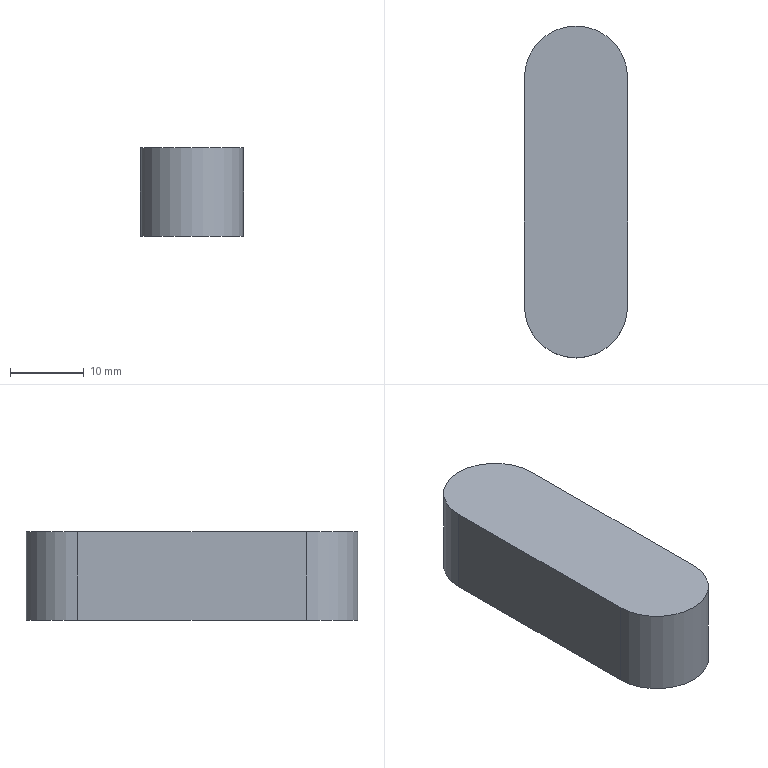Part | NX | features DATUM_CSYS 2, EXTRUDE 1, LINKED_FACE 1, SKETCH 1 | 1 solid | 6 faces | box 14 x 45 x 12 mm | volume 7055 mm3 | plane 4 | cylinder 2 | commonest cylinder face diameters 14 x2
STEP:
#1=CARTESIAN_POINT('',(35.,10.5,34.));
#2=VERTEX_POINT('',#1);
#3=CARTESIAN_POINT('',(35.,-20.5,34.));
#4=VERTEX_POINT('',#3);
#5=CARTESIAN_POINT('',(35.,10.5,34.));
#6=DIRECTION('',(0.,-1.,0.));
#7=VECTOR('',#6,1000.);
#8=LINE('',#5,#7);
#9=EDGE_CURVE('',#2,#4,#8,.T.);
#10=ORIENTED_EDGE('',*,*,#9,.T.);
#11=CARTESIAN_POINT('',(35.,-20.5,46.));
#12=VERTEX_POINT('',#11);
#13=CARTESIAN_POINT('',(35.,-20.5,46.));
#14=DIRECTION('',(0.,0.,-1.));
#15=VECTOR('',#14,1000.);
#16=LINE('',#13,#15);
#17=EDGE_CURVE('',#12,#4,#16,.T.);
#18=ORIENTED_EDGE('',*,*,#17,.F.);
#19=CARTESIAN_POINT('',(35.,10.5,46.));
#20=VERTEX_POINT('',#19);
#21=CARTESIAN_POINT('',(35.,10.5,46.));
#22=DIRECTION('',(0.,-1.,0.));
#23=VECTOR('',#22,1000.);
#24=LINE('',#21,#23);
#25=EDGE_CURVE('',#20,#12,#24,.T.);
#26=ORIENTED_EDGE('',*,*,#25,.F.);
#27=CARTESIAN_POINT('',(35.,10.5,46.));
#28=DIRECTION('',(0.,0.,-1.));
#29=VECTOR('',#28,1000.);
#30=LINE('',#27,#29);
#31=EDGE_CURVE('',#20,#2,#30,.T.);
#32=ORIENTED_EDGE('',*,*,#31,.T.);
#33=EDGE_LOOP('',(#10,#18,#26,#32));
#34=FACE_BOUND('',#33,.T.);
#35=CARTESIAN_POINT('',(35.,10.5,46.));
#36=DIRECTION('',(1.,0.,0.));
#37=DIRECTION('',(0.,1.,0.));
#38=AXIS2_PLACEMENT_3D('',#35,#36,#37);
#39=PLANE('',#38);
#40=ADVANCED_FACE('',(#34),#39,.F.);
#41=CARTESIAN_POINT('',(49.,-20.5,34.));
#42=VERTEX_POINT('',#41);
#43=CARTESIAN_POINT('',(42.,-20.5,34.));
#44=DIRECTION('',(0.,0.,1.));
#45=DIRECTION('',(-1.,0.,0.));
#46=AXIS2_PLACEMENT_3D('',#43,#44,#45);
#47=CIRCLE('',#46,7.);
#48=EDGE_CURVE('',#4,#42,#47,.T.);
#49=ORIENTED_EDGE('',*,*,#48,.T.);
#50=CARTESIAN_POINT('',(49.,-20.5,46.));
#51=VERTEX_POINT('',#50);
#52=CARTESIAN_POINT('',(49.,-20.5,46.));
#53=DIRECTION('',(0.,0.,-1.));
#54=VECTOR('',#53,1000.);
#55=LINE('',#52,#54);
#56=EDGE_CURVE('',#51,#42,#55,.T.);
#57=ORIENTED_EDGE('',*,*,#56,.F.);
#58=CARTESIAN_POINT('',(42.,-20.5,46.));
#59=DIRECTION('',(0.,0.,1.));
#60=DIRECTION('',(-1.,0.,0.));
#61=AXIS2_PLACEMENT_3D('',#58,#59,#60);
#62=CIRCLE('',#61,7.);
#63=EDGE_CURVE('',#12,#51,#62,.T.);
#64=ORIENTED_EDGE('',*,*,#63,.F.);
#65=ORIENTED_EDGE('',*,*,#17,.T.);
#66=EDGE_LOOP('',(#49,#57,#64,#65));
#67=FACE_BOUND('',#66,.T.);
#68=CARTESIAN_POINT('',(42.,-20.5,46.));
#69=DIRECTION('',(0.,0.,-1.));
#70=DIRECTION('',(-1.,0.,0.));
#71=AXIS2_PLACEMENT_3D('',#68,#69,#70);
#72=CYLINDRICAL_SURFACE('',#71,7.);
#73=ADVANCED_FACE('',(#67),#72,.T.);
#74=CARTESIAN_POINT('',(49.,10.5,34.));
#75=VERTEX_POINT('',#74);
#76=CARTESIAN_POINT('',(49.,-20.5,34.));
#77=DIRECTION('',(0.,1.,0.));
#78=VECTOR('',#77,1000.);
#79=LINE('',#76,#78);
#80=EDGE_CURVE('',#42,#75,#79,.T.);
#81=ORIENTED_EDGE('',*,*,#80,.T.);
#82=CARTESIAN_POINT('',(49.,10.5,46.));
#83=VERTEX_POINT('',#82);
#84=CARTESIAN_POINT('',(49.,10.5,46.));
#85=DIRECTION('',(0.,0.,-1.));
#86=VECTOR('',#85,1000.);
#87=LINE('',#84,#86);
#88=EDGE_CURVE('',#83,#75,#87,.T.);
#89=ORIENTED_EDGE('',*,*,#88,.F.);
#90=CARTESIAN_POINT('',(49.,-20.5,46.));
#91=DIRECTION('',(0.,1.,0.));
#92=VECTOR('',#91,1000.);
#93=LINE('',#90,#92);
#94=EDGE_CURVE('',#51,#83,#93,.T.);
#95=ORIENTED_EDGE('',*,*,#94,.F.);
#96=ORIENTED_EDGE('',*,*,#56,.T.);
#97=EDGE_LOOP('',(#81,#89,#95,#96));
#98=FACE_BOUND('',#97,.T.);
#99=CARTESIAN_POINT('',(49.,-20.5,46.));
#100=DIRECTION('',(-1.,0.,0.));
#101=DIRECTION('',(0.,-1.,0.));
#102=AXIS2_PLACEMENT_3D('',#99,#100,#101);
#103=PLANE('',#102);
#104=ADVANCED_FACE('',(#98),#103,.F.);
#105=CARTESIAN_POINT('',(42.,10.5,34.));
#106=DIRECTION('',(0.,0.,1.));
#107=DIRECTION('',(-1.,0.,0.));
#108=AXIS2_PLACEMENT_3D('',#105,#106,#107);
#109=CIRCLE('',#108,7.);
#110=EDGE_CURVE('',#75,#2,#109,.T.);
#111=ORIENTED_EDGE('',*,*,#110,.T.);
#112=ORIENTED_EDGE('',*,*,#31,.F.);
#113=CARTESIAN_POINT('',(42.,10.5,46.));
#114=DIRECTION('',(0.,0.,1.));
#115=DIRECTION('',(-1.,0.,0.));
#116=AXIS2_PLACEMENT_3D('',#113,#114,#115);
#117=CIRCLE('',#116,7.);
#118=EDGE_CURVE('',#83,#20,#117,.T.);
#119=ORIENTED_EDGE('',*,*,#118,.F.);
#120=ORIENTED_EDGE('',*,*,#88,.T.);
#121=EDGE_LOOP('',(#111,#112,#119,#120));
#122=FACE_BOUND('',#121,.T.);
#123=CARTESIAN_POINT('',(42.,10.5,46.));
#124=DIRECTION('',(0.,0.,-1.));
#125=DIRECTION('',(-1.,0.,0.));
#126=AXIS2_PLACEMENT_3D('',#123,#124,#125);
#127=CYLINDRICAL_SURFACE('',#126,7.);
#128=ADVANCED_FACE('',(#122),#127,.T.);
#129=ORIENTED_EDGE('',*,*,#25,.T.);
#130=ORIENTED_EDGE('',*,*,#63,.T.);
#131=ORIENTED_EDGE('',*,*,#94,.T.);
#132=ORIENTED_EDGE('',*,*,#118,.T.);
#133=EDGE_LOOP('',(#129,#130,#131,#132));
#134=FACE_BOUND('',#133,.T.);
#135=CARTESIAN_POINT('',(42.,-20.5,46.));
#136=DIRECTION('',(0.,0.,1.));
#137=DIRECTION('',(0.,-1.,0.));
#138=AXIS2_PLACEMENT_3D('',#135,#136,#137);
#139=PLANE('',#138);
#140=ADVANCED_FACE('',(#134),#139,.T.);
#141=ORIENTED_EDGE('',*,*,#9,.F.);
#142=ORIENTED_EDGE('',*,*,#110,.F.);
#143=ORIENTED_EDGE('',*,*,#80,.F.);
#144=ORIENTED_EDGE('',*,*,#48,.F.);
#145=EDGE_LOOP('',(#141,#142,#143,#144));
#146=FACE_BOUND('',#145,.T.);
#147=CARTESIAN_POINT('',(42.,-20.5,34.));
#148=DIRECTION('',(0.,0.,1.));
#149=DIRECTION('',(0.,-1.,0.));
#150=AXIS2_PLACEMENT_3D('',#147,#148,#149);
#151=PLANE('',#150);
#152=ADVANCED_FACE('',(#146),#151,.F.);
#153=CLOSED_SHELL('',(#40,#73,#104,#128,#140,#152));
#154=MANIFOLD_SOLID_BREP('',#153);
#155=(LENGTH_UNIT()NAMED_UNIT(*)SI_UNIT(.MILLI.,.METRE.));
#156=UNCERTAINTY_MEASURE_WITH_UNIT(LENGTH_MEASURE(0.00001),#155,'','');
#157=(NAMED_UNIT(*)PLANE_ANGLE_UNIT()SI_UNIT($,.RADIAN.));
#158=(NAMED_UNIT(*)SI_UNIT($,.STERADIAN.)SOLID_ANGLE_UNIT());
#159=(GEOMETRIC_REPRESENTATION_CONTEXT(3)GLOBAL_UNCERTAINTY_ASSIGNED_CONTEXT((#156))GLOBAL_UNIT_ASSIGNED_CONTEXT((#155,#157,#158))REPRESENTATION_CONTEXT('',''));
#160=ADVANCED_BREP_SHAPE_REPRESENTATION('',(#154),#159);